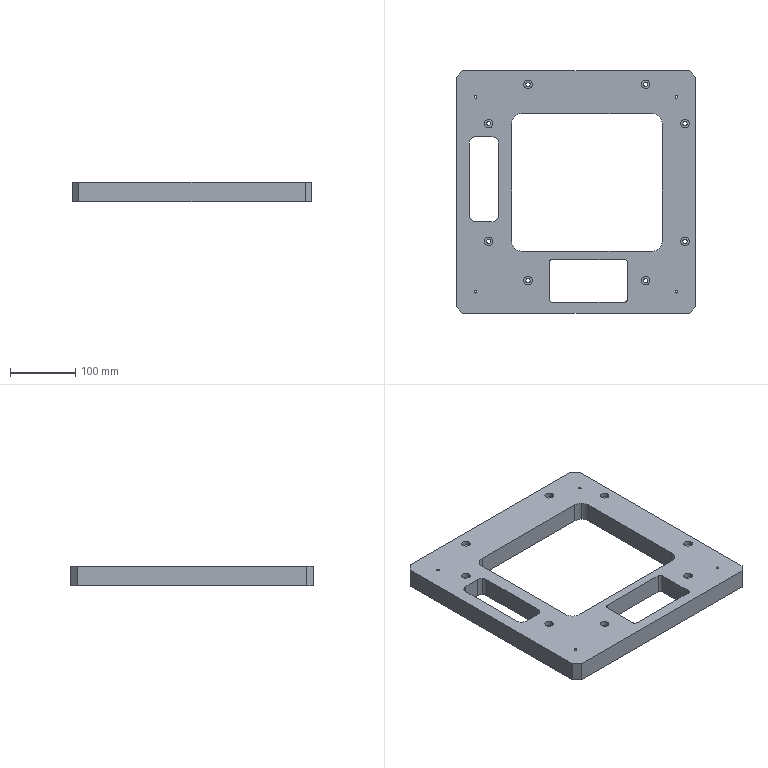Part | STEP file | ASND-0110-Body 1-13 | 1 solid | 90 faces | box 366.812 x 370.85 x 30 mm | volume 2210329 mm3 | cylinder 60 | plane 30 | commonest cylinder face diameters 6.5 x16 13 x16 4.134 x8 20 x8 30 x8 10 x4